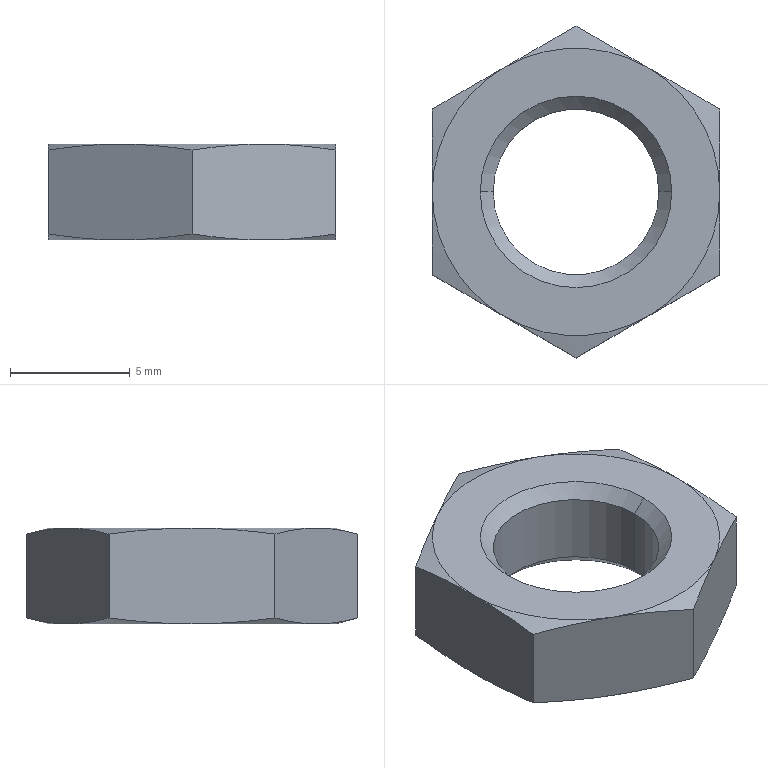Part | SolidWorks | features BaseBody 1 | 1 solid | 26 faces | box 12 x 13.856 x 4 mm | volume 340.073 mm3 | cone 16 | plane 8 | cylinder 2 | commonest cylinder face diameters 6.917 x2
STEP:
#1=CARTESIAN_POINT('',(3.459,0.,0.5415));
#2=VERTEX_POINT('',#1);
#3=CARTESIAN_POINT('',(-3.459,0.,0.5415));
#4=VERTEX_POINT('',#3);
#5=CARTESIAN_POINT('',(0.,0.,0.5415));
#6=DIRECTION('',(0.,0.,-1.));
#7=DIRECTION('',(-1.,0.,0.));
#8=AXIS2_PLACEMENT_3D('',#5,#6,#7);
#9=CIRCLE('',#8,3.459);
#10=EDGE_CURVE('',#2,#4,#9,.T.);
#11=ORIENTED_EDGE('',*,*,#10,.F.);
#12=CARTESIAN_POINT('',(4.,0.,0.));
#13=VERTEX_POINT('',#12);
#14=CARTESIAN_POINT('',(3.459,0.,0.5415));
#15=DIRECTION('',(0.7071,0.,-0.7071));
#16=VECTOR('',#15,1000.);
#17=LINE('',#14,#16);
#18=EDGE_CURVE('',#2,#13,#17,.T.);
#19=ORIENTED_EDGE('',*,*,#18,.T.);
#20=CARTESIAN_POINT('',(-4.,0.,0.));
#21=VERTEX_POINT('',#20);
#22=CARTESIAN_POINT('',(0.,0.,0.));
#23=DIRECTION('',(0.,0.,-1.));
#24=DIRECTION('',(-1.,0.,0.));
#25=AXIS2_PLACEMENT_3D('',#22,#23,#24);
#26=CIRCLE('',#25,4.);
#27=EDGE_CURVE('',#13,#21,#26,.T.);
#28=ORIENTED_EDGE('',*,*,#27,.T.);
#29=CARTESIAN_POINT('',(-3.459,0.,0.5415));
#30=DIRECTION('',(-0.7071,0.,-0.7071));
#31=VECTOR('',#30,1000.);
#32=LINE('',#29,#31);
#33=EDGE_CURVE('',#4,#21,#32,.T.);
#34=ORIENTED_EDGE('',*,*,#33,.F.);
#35=EDGE_LOOP('',(#11,#19,#28,#34));
#36=FACE_OUTER_BOUND('',#35,.T.);
#37=CARTESIAN_POINT('',(0.,0.,0.5415));
#38=DIRECTION('',(0.,0.,-1.));
#39=DIRECTION('',(-1.,0.,0.));
#40=AXIS2_PLACEMENT_3D('',#37,#38,#39);
#41=CONICAL_SURFACE('',#40,3.459,0.7854);
#42=ADVANCED_FACE('',(#36),#41,.F.);
#43=CARTESIAN_POINT('',(3.459,0.,3.459));
#44=VERTEX_POINT('',#43);
#45=CARTESIAN_POINT('',(-3.459,0.,3.459));
#46=VERTEX_POINT('',#45);
#47=CARTESIAN_POINT('',(0.,0.,3.459));
#48=DIRECTION('',(0.,0.,-1.));
#49=DIRECTION('',(-1.,0.,0.));
#50=AXIS2_PLACEMENT_3D('',#47,#48,#49);
#51=CIRCLE('',#50,3.459);
#52=EDGE_CURVE('',#44,#46,#51,.T.);
#53=ORIENTED_EDGE('',*,*,#52,.F.);
#54=CARTESIAN_POINT('',(3.459,0.,0.));
#55=DIRECTION('',(0.,0.,-1.));
#56=VECTOR('',#55,1000.);
#57=LINE('',#54,#56);
#58=EDGE_CURVE('',#44,#2,#57,.T.);
#59=ORIENTED_EDGE('',*,*,#58,.T.);
#60=ORIENTED_EDGE('',*,*,#10,.T.);
#61=CARTESIAN_POINT('',(-3.459,0.,0.));
#62=DIRECTION('',(0.,0.,-1.));
#63=VECTOR('',#62,1000.);
#64=LINE('',#61,#63);
#65=EDGE_CURVE('',#46,#4,#64,.T.);
#66=ORIENTED_EDGE('',*,*,#65,.F.);
#67=EDGE_LOOP('',(#53,#59,#60,#66));
#68=FACE_OUTER_BOUND('',#67,.T.);
#69=CARTESIAN_POINT('',(0.,0.,0.));
#70=DIRECTION('',(0.,0.,-1.));
#71=DIRECTION('',(-1.,0.,0.));
#72=AXIS2_PLACEMENT_3D('',#69,#70,#71);
#73=CYLINDRICAL_SURFACE('',#72,3.459);
#74=ADVANCED_FACE('',(#68),#73,.F.);
#75=ORIENTED_EDGE('',*,*,#52,.T.);
#76=CARTESIAN_POINT('',(-4.,0.,4.));
#77=VERTEX_POINT('',#76);
#78=CARTESIAN_POINT('',(-4.,0.,4.));
#79=DIRECTION('',(-0.7071,0.,0.7071));
#80=VECTOR('',#79,1000.);
#81=LINE('',#78,#80);
#82=EDGE_CURVE('',#46,#77,#81,.T.);
#83=ORIENTED_EDGE('',*,*,#82,.T.);
#84=CARTESIAN_POINT('',(4.,0.,4.));
#85=VERTEX_POINT('',#84);
#86=CARTESIAN_POINT('',(0.,0.,4.));
#87=DIRECTION('',(0.,0.,-1.));
#88=DIRECTION('',(-1.,0.,0.));
#89=AXIS2_PLACEMENT_3D('',#86,#87,#88);
#90=CIRCLE('',#89,4.);
#91=EDGE_CURVE('',#85,#77,#90,.T.);
#92=ORIENTED_EDGE('',*,*,#91,.F.);
#93=CARTESIAN_POINT('',(4.,0.,4.));
#94=DIRECTION('',(0.7071,0.,0.7071));
#95=VECTOR('',#94,1000.);
#96=LINE('',#93,#95);
#97=EDGE_CURVE('',#44,#85,#96,.T.);
#98=ORIENTED_EDGE('',*,*,#97,.F.);
#99=EDGE_LOOP('',(#75,#83,#92,#98));
#100=FACE_OUTER_BOUND('',#99,.T.);
#101=CARTESIAN_POINT('',(0.,0.,4.));
#102=DIRECTION('',(0.,0.,1.));
#103=DIRECTION('',(1.,0.,0.));
#104=AXIS2_PLACEMENT_3D('',#101,#102,#103);
#105=CONICAL_SURFACE('',#104,4.,0.7854);
#106=ADVANCED_FACE('',(#100),#105,.F.);
#107=CARTESIAN_POINT('',(-6.,-3.464,3.751));
#108=VERTEX_POINT('',#107);
#109=CARTESIAN_POINT('',(-6.,0.,4.));
#110=VERTEX_POINT('',#109);
#111=CARTESIAN_POINT('',(-6.,-3.464,3.751));
#112=CARTESIAN_POINT('',(-6.,-2.891,3.828));
#113=CARTESIAN_POINT('',(-6.,-2.318,3.891));
#114=CARTESIAN_POINT('',(-6.,-1.162,3.977));
#115=CARTESIAN_POINT('',(-6.,-0.5807,4.));
#116=CARTESIAN_POINT('',(-6.,0.,4.));
#117=B_SPLINE_CURVE_WITH_KNOTS('',3,(#111,#112,#113,#114,#115,#116),.UNSPECIFIED.,.F.,.F.,(4,2,4),(7.335,9.068,10.801),.UNSPECIFIED.);
#118=EDGE_CURVE('',#108,#110,#117,.T.);
#119=ORIENTED_EDGE('',*,*,#118,.F.);
#120=CARTESIAN_POINT('',(-3.,-5.196,4.));
#121=VERTEX_POINT('',#120);
#122=CARTESIAN_POINT('',(-3.,-5.196,4.));
#123=CARTESIAN_POINT('',(-3.501,-4.907,4.));
#124=CARTESIAN_POINT('',(-4.,-4.619,3.977));
#125=CARTESIAN_POINT('',(-5.001,-4.041,3.891));
#126=CARTESIAN_POINT('',(-5.502,-3.752,3.828));
#127=CARTESIAN_POINT('',(-6.,-3.464,3.751));
#128=B_SPLINE_CURVE_WITH_KNOTS('',3,(#122,#123,#124,#125,#126,#127),.UNSPECIFIED.,.F.,.F.,(4,2,4),(3.464,5.196,6.928),.UNSPECIFIED.);
#129=EDGE_CURVE('',#121,#108,#128,.T.);
#130=ORIENTED_EDGE('',*,*,#129,.F.);
#131=CARTESIAN_POINT('',(0.,0.,4.));
#132=DIRECTION('',(0.,0.,-1.));
#133=DIRECTION('',(-0.5,-0.866,0.));
#134=AXIS2_PLACEMENT_3D('',#131,#132,#133);
#135=CIRCLE('',#134,6.);
#136=EDGE_CURVE('',#121,#110,#135,.T.);
#137=ORIENTED_EDGE('',*,*,#136,.T.);
#138=EDGE_LOOP('',(#119,#130,#137));
#139=FACE_OUTER_BOUND('',#138,.T.);
#140=CARTESIAN_POINT('',(0.,0.,2.));
#141=DIRECTION('',(0.,0.,-1.));
#142=DIRECTION('',(-1.,0.,0.));
#143=AXIS2_PLACEMENT_3D('',#140,#141,#142);
#144=CONICAL_SURFACE('',#143,13.464,1.309);
#145=ADVANCED_FACE('',(#139),#144,.T.);
#146=ORIENTED_EDGE('',*,*,#118,.T.);
#147=CARTESIAN_POINT('',(-6.,3.464,3.751));
#148=VERTEX_POINT('',#147);
#149=CARTESIAN_POINT('',(-6.,0.,4.));
#150=CARTESIAN_POINT('',(-6.,0.5782,4.));
#151=CARTESIAN_POINT('',(-6.,1.154,3.977));
#152=CARTESIAN_POINT('',(-6.,2.31,3.891));
#153=CARTESIAN_POINT('',(-6.,2.889,3.828));
#154=CARTESIAN_POINT('',(-6.,3.464,3.751));
#155=B_SPLINE_CURVE_WITH_KNOTS('',3,(#149,#150,#151,#152,#153,#154),.UNSPECIFIED.,.F.,.F.,(4,2,4),(10.801,12.511,14.221),.UNSPECIFIED.);
#156=EDGE_CURVE('',#110,#148,#155,.T.);
#157=ORIENTED_EDGE('',*,*,#156,.T.);
#158=CARTESIAN_POINT('',(-6.,3.464,0.2487));
#159=VERTEX_POINT('',#158);
#160=CARTESIAN_POINT('',(-6.,3.464,3.751));
#161=DIRECTION('',(0.,0.,-1.));
#162=VECTOR('',#161,1000.);
#163=LINE('',#160,#162);
#164=EDGE_CURVE('',#148,#159,#163,.T.);
#165=ORIENTED_EDGE('',*,*,#164,.T.);
#166=CARTESIAN_POINT('',(-6.,0.,0.));
#167=VERTEX_POINT('',#166);
#168=CARTESIAN_POINT('',(-6.,3.464,0.2487));
#169=CARTESIAN_POINT('',(-6.,2.891,0.1719));
#170=CARTESIAN_POINT('',(-6.,2.318,0.1093));
#171=CARTESIAN_POINT('',(-6.,1.162,0.0231));
#172=CARTESIAN_POINT('',(-6.,0.5807,0.00000014));
#173=CARTESIAN_POINT('',(-6.,0.,0.));
#174=B_SPLINE_CURVE_WITH_KNOTS('',3,(#168,#169,#170,#171,#172,#173),.UNSPECIFIED.,.F.,.F.,(4,2,4),(7.335,9.068,10.801),.UNSPECIFIED.);
#175=EDGE_CURVE('',#159,#167,#174,.T.);
#176=ORIENTED_EDGE('',*,*,#175,.T.);
#177=CARTESIAN_POINT('',(-6.,-3.464,0.2487));
#178=VERTEX_POINT('',#177);
#179=CARTESIAN_POINT('',(-6.,0.,0.));
#180=CARTESIAN_POINT('',(-6.,-0.5782,-0.00000014));
#181=CARTESIAN_POINT('',(-6.,-1.154,0.02271));
#182=CARTESIAN_POINT('',(-6.,-2.31,0.1086));
#183=CARTESIAN_POINT('',(-6.,-2.889,0.1716));
#184=CARTESIAN_POINT('',(-6.,-3.464,0.2487));
#185=B_SPLINE_CURVE_WITH_KNOTS('',3,(#179,#180,#181,#182,#183,#184),.UNSPECIFIED.,.F.,.F.,(4,2,4),(10.801,12.511,14.221),.UNSPECIFIED.);
#186=EDGE_CURVE('',#167,#178,#185,.T.);
#187=ORIENTED_EDGE('',*,*,#186,.T.);
#188=CARTESIAN_POINT('',(-6.,-3.464,3.751));
#189=DIRECTION('',(0.,0.,-1.));
#190=VECTOR('',#189,1000.);
#191=LINE('',#188,#190);
#192=EDGE_CURVE('',#108,#178,#191,.T.);
#193=ORIENTED_EDGE('',*,*,#192,.F.);
#194=EDGE_LOOP('',(#146,#157,#165,#176,#187,#193));
#195=FACE_OUTER_BOUND('',#194,.T.);
#196=CARTESIAN_POINT('',(-6.,3.464,4.));
#197=DIRECTION('',(1.,0.,0.));
#198=DIRECTION('',(0.,0.,-1.));
#199=AXIS2_PLACEMENT_3D('',#196,#197,#198);
#200=PLANE('',#199);
#201=ADVANCED_FACE('',(#195),#200,.F.);
#202=CARTESIAN_POINT('',(0.,-6.928,3.751));
#203=VERTEX_POINT('',#202);
#204=CARTESIAN_POINT('',(0.,-6.928,3.751));
#205=CARTESIAN_POINT('',(-0.4983,-6.64,3.828));
#206=CARTESIAN_POINT('',(-0.9989,-6.351,3.891));
#207=CARTESIAN_POINT('',(-2.,-5.774,3.977));
#208=CARTESIAN_POINT('',(-2.499,-5.485,4.));
#209=CARTESIAN_POINT('',(-3.,-5.196,4.));
#210=B_SPLINE_CURVE_WITH_KNOTS('',3,(#204,#205,#206,#207,#208,#209),.UNSPECIFIED.,.F.,.F.,(4,2,4),(0.0002309,1.732,3.464),.UNSPECIFIED.);
#211=EDGE_CURVE('',#203,#121,#210,.T.);
#212=ORIENTED_EDGE('',*,*,#211,.T.);
#213=ORIENTED_EDGE('',*,*,#129,.T.);
#214=ORIENTED_EDGE('',*,*,#192,.T.);
#215=CARTESIAN_POINT('',(-3.,-5.196,0.));
#216=VERTEX_POINT('',#215);
#217=CARTESIAN_POINT('',(-6.,-3.464,0.2487));
#218=CARTESIAN_POINT('',(-5.502,-3.752,0.1716));
#219=CARTESIAN_POINT('',(-5.001,-4.041,0.1087));
#220=CARTESIAN_POINT('',(-4.,-4.619,0.02273));
#221=CARTESIAN_POINT('',(-3.501,-4.907,0.));
#222=CARTESIAN_POINT('',(-3.,-5.196,0.));
#223=B_SPLINE_CURVE_WITH_KNOTS('',3,(#217,#218,#219,#220,#221,#222),.UNSPECIFIED.,.F.,.F.,(4,2,4),(0.0002309,1.732,3.464),.UNSPECIFIED.);
#224=EDGE_CURVE('',#178,#216,#223,.T.);
#225=ORIENTED_EDGE('',*,*,#224,.T.);
#226=CARTESIAN_POINT('',(0.,-6.928,0.2487));
#227=VERTEX_POINT('',#226);
#228=CARTESIAN_POINT('',(-3.,-5.196,0.));
#229=CARTESIAN_POINT('',(-2.499,-5.485,0.));
#230=CARTESIAN_POINT('',(-2.,-5.774,0.02273));
#231=CARTESIAN_POINT('',(-0.9989,-6.351,0.1087));
#232=CARTESIAN_POINT('',(-0.4983,-6.64,0.1716));
#233=CARTESIAN_POINT('',(0.,-6.928,0.2487));
#234=B_SPLINE_CURVE_WITH_KNOTS('',3,(#228,#229,#230,#231,#232,#233),.UNSPECIFIED.,.F.,.F.,(4,2,4),(3.464,5.196,6.928),.UNSPECIFIED.);
#235=EDGE_CURVE('',#216,#227,#234,.T.);
#236=ORIENTED_EDGE('',*,*,#235,.T.);
#237=CARTESIAN_POINT('',(0.,-6.928,3.751));
#238=DIRECTION('',(0.,0.,-1.));
#239=VECTOR('',#238,1000.);
#240=LINE('',#237,#239);
#241=EDGE_CURVE('',#203,#227,#240,.T.);
#242=ORIENTED_EDGE('',*,*,#241,.F.);
#243=EDGE_LOOP('',(#212,#213,#214,#225,#236,#242));
#244=FACE_OUTER_BOUND('',#243,.T.);
#245=CARTESIAN_POINT('',(-6.,-3.464,4.));
#246=DIRECTION('',(0.5,0.866,0.));
#247=DIRECTION('',(-0.866,0.5,0.));
#248=AXIS2_PLACEMENT_3D('',#245,#246,#247);
#249=PLANE('',#248);
#250=ADVANCED_FACE('',(#244),#249,.F.);
#251=ORIENTED_EDGE('',*,*,#91,.T.);
#252=CARTESIAN_POINT('',(0.,0.,4.));
#253=DIRECTION('',(0.,0.,-1.));
#254=DIRECTION('',(-1.,0.,0.));
#255=AXIS2_PLACEMENT_3D('',#252,#253,#254);
#256=CIRCLE('',#255,4.);
#257=EDGE_CURVE('',#77,#85,#256,.T.);
#258=ORIENTED_EDGE('',*,*,#257,.T.);
#259=EDGE_LOOP('',(#251,#258));
#260=FACE_BOUND('',#259,.T.);
#261=CARTESIAN_POINT('',(-3.,5.196,4.));
#262=VERTEX_POINT('',#261);
#263=CARTESIAN_POINT('',(3.,5.196,4.));
#264=VERTEX_POINT('',#263);
#265=CARTESIAN_POINT('',(0.,0.,4.));
#266=DIRECTION('',(0.,0.,-1.));
#267=DIRECTION('',(-0.5,0.866,0.));
#268=AXIS2_PLACEMENT_3D('',#265,#266,#267);
#269=CIRCLE('',#268,6.);
#270=EDGE_CURVE('',#262,#264,#269,.T.);
#271=ORIENTED_EDGE('',*,*,#270,.F.);
#272=CARTESIAN_POINT('',(0.,0.,4.));
#273=DIRECTION('',(0.,0.,-1.));
#274=DIRECTION('',(-1.,0.,0.));
#275=AXIS2_PLACEMENT_3D('',#272,#273,#274);
#276=CIRCLE('',#275,6.);
#277=EDGE_CURVE('',#110,#262,#276,.T.);
#278=ORIENTED_EDGE('',*,*,#277,.F.);
#279=ORIENTED_EDGE('',*,*,#136,.F.);
#280=CARTESIAN_POINT('',(3.,-5.196,4.));
#281=VERTEX_POINT('',#280);
#282=CARTESIAN_POINT('',(0.,0.,4.));
#283=DIRECTION('',(0.,0.,-1.));
#284=DIRECTION('',(0.5,-0.866,0.));
#285=AXIS2_PLACEMENT_3D('',#282,#283,#284);
#286=CIRCLE('',#285,6.);
#287=EDGE_CURVE('',#281,#121,#286,.T.);
#288=ORIENTED_EDGE('',*,*,#287,.F.);
#289=CARTESIAN_POINT('',(6.,0.,4.));
#290=VERTEX_POINT('',#289);
#291=CARTESIAN_POINT('',(0.,0.,4.));
#292=DIRECTION('',(0.,0.,-1.));
#293=DIRECTION('',(1.,0.,0.));
#294=AXIS2_PLACEMENT_3D('',#291,#292,#293);
#295=CIRCLE('',#294,6.);
#296=EDGE_CURVE('',#290,#281,#295,.T.);
#297=ORIENTED_EDGE('',*,*,#296,.F.);
#298=CARTESIAN_POINT('',(0.,0.,4.));
#299=DIRECTION('',(0.,0.,-1.));
#300=DIRECTION('',(0.5,0.866,0.));
#301=AXIS2_PLACEMENT_3D('',#298,#299,#300);
#302=CIRCLE('',#301,6.);
#303=EDGE_CURVE('',#264,#290,#302,.T.);
#304=ORIENTED_EDGE('',*,*,#303,.F.);
#305=EDGE_LOOP('',(#271,#278,#279,#288,#297,#304));
#306=FACE_OUTER_BOUND('',#305,.T.);
#307=CARTESIAN_POINT('',(0.,6.,4.));
#308=DIRECTION('',(0.,0.,1.));
#309=DIRECTION('',(1.,0.,0.));
#310=AXIS2_PLACEMENT_3D('',#307,#308,#309);
#311=PLANE('',#310);
#312=ADVANCED_FACE('',(#260,#306),#311,.T.);
#313=ORIENTED_EDGE('',*,*,#156,.F.);
#314=ORIENTED_EDGE('',*,*,#277,.T.);
#315=CARTESIAN_POINT('',(-6.,3.464,3.751));
#316=CARTESIAN_POINT('',(-5.502,3.752,3.828));
#317=CARTESIAN_POINT('',(-5.001,4.041,3.891));
#318=CARTESIAN_POINT('',(-4.,4.619,3.977));
#319=CARTESIAN_POINT('',(-3.501,4.907,4.));
#320=CARTESIAN_POINT('',(-3.,5.196,4.));
#321=B_SPLINE_CURVE_WITH_KNOTS('',3,(#315,#316,#317,#318,#319,#320),.UNSPECIFIED.,.F.,.F.,(4,2,4),(0.0002309,1.732,3.464),.UNSPECIFIED.);
#322=EDGE_CURVE('',#148,#262,#321,.T.);
#323=ORIENTED_EDGE('',*,*,#322,.F.);
#324=EDGE_LOOP('',(#313,#314,#323));
#325=FACE_OUTER_BOUND('',#324,.T.);
#326=CARTESIAN_POINT('',(0.,0.,2.));
#327=DIRECTION('',(0.,0.,-1.));
#328=DIRECTION('',(-1.,0.,0.));
#329=AXIS2_PLACEMENT_3D('',#326,#327,#328);
#330=CONICAL_SURFACE('',#329,13.464,1.309);
#331=ADVANCED_FACE('',(#325),#330,.T.);
#332=ORIENTED_EDGE('',*,*,#322,.T.);
#333=CARTESIAN_POINT('',(0.,6.928,3.751));
#334=VERTEX_POINT('',#333);
#335=CARTESIAN_POINT('',(-3.,5.196,4.));
#336=CARTESIAN_POINT('',(-2.499,5.485,4.));
#337=CARTESIAN_POINT('',(-2.,5.774,3.977));
#338=CARTESIAN_POINT('',(-0.9989,6.351,3.891));
#339=CARTESIAN_POINT('',(-0.4983,6.64,3.828));
#340=CARTESIAN_POINT('',(0.,6.928,3.751));
#341=B_SPLINE_CURVE_WITH_KNOTS('',3,(#335,#336,#337,#338,#339,#340),.UNSPECIFIED.,.F.,.F.,(4,2,4),(3.464,5.196,6.928),.UNSPECIFIED.);
#342=EDGE_CURVE('',#262,#334,#341,.T.);
#343=ORIENTED_EDGE('',*,*,#342,.T.);
#344=CARTESIAN_POINT('',(0.,6.928,0.2487));
#345=VERTEX_POINT('',#344);
#346=CARTESIAN_POINT('',(0.,6.928,3.751));
#347=DIRECTION('',(0.,0.,-1.));
#348=VECTOR('',#347,1000.);
#349=LINE('',#346,#348);
#350=EDGE_CURVE('',#334,#345,#349,.T.);
#351=ORIENTED_EDGE('',*,*,#350,.T.);
#352=CARTESIAN_POINT('',(-3.,5.196,0.));
#353=VERTEX_POINT('',#352);
#354=CARTESIAN_POINT('',(0.,6.928,0.2487));
#355=CARTESIAN_POINT('',(-0.4983,6.64,0.1716));
#356=CARTESIAN_POINT('',(-0.9989,6.351,0.1087));
#357=CARTESIAN_POINT('',(-2.,5.774,0.02273));
#358=CARTESIAN_POINT('',(-2.499,5.485,0.));
#359=CARTESIAN_POINT('',(-3.,5.196,0.));
#360=B_SPLINE_CURVE_WITH_KNOTS('',3,(#354,#355,#356,#357,#358,#359),.UNSPECIFIED.,.F.,.F.,(4,2,4),(0.0002309,1.732,3.464),.UNSPECIFIED.);
#361=EDGE_CURVE('',#345,#353,#360,.T.);
#362=ORIENTED_EDGE('',*,*,#361,.T.);
#363=CARTESIAN_POINT('',(-3.,5.196,0.));
#364=CARTESIAN_POINT('',(-3.501,4.907,0.));
#365=CARTESIAN_POINT('',(-4.,4.619,0.02273));
#366=CARTESIAN_POINT('',(-5.001,4.041,0.1087));
#367=CARTESIAN_POINT('',(-5.502,3.752,0.1716));
#368=CARTESIAN_POINT('',(-6.,3.464,0.2487));
#369=B_SPLINE_CURVE_WITH_KNOTS('',3,(#363,#364,#365,#366,#367,#368),.UNSPECIFIED.,.F.,.F.,(4,2,4),(3.464,5.196,6.928),.UNSPECIFIED.);
#370=EDGE_CURVE('',#353,#159,#369,.T.);
#371=ORIENTED_EDGE('',*,*,#370,.T.);
#372=ORIENTED_EDGE('',*,*,#164,.F.);
#373=EDGE_LOOP('',(#332,#343,#351,#362,#371,#372));
#374=FACE_OUTER_BOUND('',#373,.T.);
#375=CARTESIAN_POINT('',(0.,6.928,4.));
#376=DIRECTION('',(0.5,-0.866,0.));
#377=DIRECTION('',(0.866,0.5,0.));
#378=AXIS2_PLACEMENT_3D('',#375,#376,#377);
#379=PLANE('',#378);
#380=ADVANCED_FACE('',(#374),#379,.F.);
#381=ORIENTED_EDGE('',*,*,#370,.F.);
#382=CARTESIAN_POINT('',(0.,0.,0.));
#383=DIRECTION('',(0.,0.,-1.));
#384=DIRECTION('',(-1.,0.,0.));
#385=AXIS2_PLACEMENT_3D('',#382,#383,#384);
#386=CIRCLE('',#385,6.);
#387=EDGE_CURVE('',#167,#353,#386,.T.);
#388=ORIENTED_EDGE('',*,*,#387,.F.);
#389=ORIENTED_EDGE('',*,*,#175,.F.);
#390=EDGE_LOOP('',(#381,#388,#389));
#391=FACE_OUTER_BOUND('',#390,.T.);
#392=CARTESIAN_POINT('',(0.,0.,0.));
#393=DIRECTION('',(0.,0.,1.));
#394=DIRECTION('',(1.,0.,0.));
#395=AXIS2_PLACEMENT_3D('',#392,#393,#394);
#396=CONICAL_SURFACE('',#395,6.,1.309);
#397=ADVANCED_FACE('',(#391),#396,.T.);
#398=ORIENTED_EDGE('',*,*,#186,.F.);
#399=CARTESIAN_POINT('',(0.,0.,0.));
#400=DIRECTION('',(0.,0.,-1.));
#401=DIRECTION('',(-0.5,-0.866,0.));
#402=AXIS2_PLACEMENT_3D('',#399,#400,#401);
#403=CIRCLE('',#402,6.);
#404=EDGE_CURVE('',#216,#167,#403,.T.);
#405=ORIENTED_EDGE('',*,*,#404,.F.);
#406=ORIENTED_EDGE('',*,*,#224,.F.);
#407=EDGE_LOOP('',(#398,#405,#406));
#408=FACE_OUTER_BOUND('',#407,.T.);
#409=CARTESIAN_POINT('',(0.,0.,0.));
#410=DIRECTION('',(0.,0.,1.));
#411=DIRECTION('',(1.,0.,0.));
#412=AXIS2_PLACEMENT_3D('',#409,#410,#411);
#413=CONICAL_SURFACE('',#412,6.,1.309);
#414=ADVANCED_FACE('',(#408),#413,.T.);
#415=CARTESIAN_POINT('',(3.,-5.196,4.));
#416=CARTESIAN_POINT('',(2.499,-5.485,4.));
#417=CARTESIAN_POINT('',(2.,-5.774,3.977));
#418=CARTESIAN_POINT('',(0.9989,-6.351,3.891));
#419=CARTESIAN_POINT('',(0.4983,-6.64,3.828));
#420=CARTESIAN_POINT('',(0.,-6.928,3.751));
#421=B_SPLINE_CURVE_WITH_KNOTS('',3,(#415,#416,#417,#418,#419,#420),.UNSPECIFIED.,.F.,.F.,(4,2,4),(3.464,5.196,6.928),.UNSPECIFIED.);
#422=EDGE_CURVE('',#281,#203,#421,.T.);
#423=ORIENTED_EDGE('',*,*,#422,.F.);
#424=ORIENTED_EDGE('',*,*,#287,.T.);
#425=ORIENTED_EDGE('',*,*,#211,.F.);
#426=EDGE_LOOP('',(#423,#424,#425));
#427=FACE_OUTER_BOUND('',#426,.T.);
#428=CARTESIAN_POINT('',(0.,0.,2.));
#429=DIRECTION('',(0.,0.,-1.));
#430=DIRECTION('',(-1.,0.,0.));
#431=AXIS2_PLACEMENT_3D('',#428,#429,#430);
#432=CONICAL_SURFACE('',#431,13.464,1.309);
#433=ADVANCED_FACE('',(#427),#432,.T.);
#434=CARTESIAN_POINT('',(3.,-5.196,0.));
#435=VERTEX_POINT('',#434);
#436=CARTESIAN_POINT('',(0.,-6.928,0.2487));
#437=CARTESIAN_POINT('',(0.4983,-6.64,0.1716));
#438=CARTESIAN_POINT('',(0.9989,-6.351,0.1087));
#439=CARTESIAN_POINT('',(2.,-5.774,0.02273));
#440=CARTESIAN_POINT('',(2.499,-5.485,0.));
#441=CARTESIAN_POINT('',(3.,-5.196,0.));
#442=B_SPLINE_CURVE_WITH_KNOTS('',3,(#436,#437,#438,#439,#440,#441),.UNSPECIFIED.,.F.,.F.,(4,2,4),(0.0002309,1.732,3.464),.UNSPECIFIED.);
#443=EDGE_CURVE('',#227,#435,#442,.T.);
#444=ORIENTED_EDGE('',*,*,#443,.F.);
#445=ORIENTED_EDGE('',*,*,#235,.F.);
#446=CARTESIAN_POINT('',(0.,0.,0.));
#447=DIRECTION('',(0.,0.,-1.));
#448=DIRECTION('',(0.5,-0.866,0.));
#449=AXIS2_PLACEMENT_3D('',#446,#447,#448);
#450=CIRCLE('',#449,6.);
#451=EDGE_CURVE('',#435,#216,#450,.T.);
#452=ORIENTED_EDGE('',*,*,#451,.F.);
#453=EDGE_LOOP('',(#444,#445,#452));
#454=FACE_OUTER_BOUND('',#453,.T.);
#455=CARTESIAN_POINT('',(0.,0.,0.));
#456=DIRECTION('',(0.,0.,1.));
#457=DIRECTION('',(1.,0.,0.));
#458=AXIS2_PLACEMENT_3D('',#455,#456,#457);
#459=CONICAL_SURFACE('',#458,6.,1.309);
#460=ADVANCED_FACE('',(#454),#459,.T.);
#461=CARTESIAN_POINT('',(6.,-3.464,3.751));
#462=VERTEX_POINT('',#461);
#463=CARTESIAN_POINT('',(6.,-3.464,3.751));
#464=CARTESIAN_POINT('',(5.502,-3.752,3.828));
#465=CARTESIAN_POINT('',(5.001,-4.041,3.891));
#466=CARTESIAN_POINT('',(4.,-4.619,3.977));
#467=CARTESIAN_POINT('',(3.501,-4.907,4.));
#468=CARTESIAN_POINT('',(3.,-5.196,4.));
#469=B_SPLINE_CURVE_WITH_KNOTS('',3,(#463,#464,#465,#466,#467,#468),.UNSPECIFIED.,.F.,.F.,(4,2,4),(0.0002309,1.732,3.464),.UNSPECIFIED.);
#470=EDGE_CURVE('',#462,#281,#469,.T.);
#471=ORIENTED_EDGE('',*,*,#470,.T.);
#472=ORIENTED_EDGE('',*,*,#422,.T.);
#473=ORIENTED_EDGE('',*,*,#241,.T.);
#474=ORIENTED_EDGE('',*,*,#443,.T.);
#475=CARTESIAN_POINT('',(6.,-3.464,0.2487));
#476=VERTEX_POINT('',#475);
#477=CARTESIAN_POINT('',(3.,-5.196,0.));
#478=CARTESIAN_POINT('',(3.501,-4.907,0.));
#479=CARTESIAN_POINT('',(4.,-4.619,0.02273));
#480=CARTESIAN_POINT('',(5.001,-4.041,0.1087));
#481=CARTESIAN_POINT('',(5.502,-3.752,0.1716));
#482=CARTESIAN_POINT('',(6.,-3.464,0.2487));
#483=B_SPLINE_CURVE_WITH_KNOTS('',3,(#477,#478,#479,#480,#481,#482),.UNSPECIFIED.,.F.,.F.,(4,2,4),(3.464,5.196,6.928),.UNSPECIFIED.);
#484=EDGE_CURVE('',#435,#476,#483,.T.);
#485=ORIENTED_EDGE('',*,*,#484,.T.);
#486=CARTESIAN_POINT('',(6.,-3.464,3.751));
#487=DIRECTION('',(0.,0.,-1.));
#488=VECTOR('',#487,1000.);
#489=LINE('',#486,#488);
#490=EDGE_CURVE('',#462,#476,#489,.T.);
#491=ORIENTED_EDGE('',*,*,#490,.F.);
#492=EDGE_LOOP('',(#471,#472,#473,#474,#485,#491));
#493=FACE_OUTER_BOUND('',#492,.T.);
#494=CARTESIAN_POINT('',(0.,-6.928,4.));
#495=DIRECTION('',(-0.5,0.866,0.));
#496=DIRECTION('',(-0.866,-0.5,0.));
#497=AXIS2_PLACEMENT_3D('',#494,#495,#496);
#498=PLANE('',#497);
#499=ADVANCED_FACE('',(#493),#498,.F.);
#500=ORIENTED_EDGE('',*,*,#82,.F.);
#501=CARTESIAN_POINT('',(0.,0.,3.459));
#502=DIRECTION('',(0.,0.,-1.));
#503=DIRECTION('',(-1.,0.,0.));
#504=AXIS2_PLACEMENT_3D('',#501,#502,#503);
#505=CIRCLE('',#504,3.459);
#506=EDGE_CURVE('',#46,#44,#505,.T.);
#507=ORIENTED_EDGE('',*,*,#506,.T.);
#508=ORIENTED_EDGE('',*,*,#97,.T.);
#509=ORIENTED_EDGE('',*,*,#257,.F.);
#510=EDGE_LOOP('',(#500,#507,#508,#509));
#511=FACE_OUTER_BOUND('',#510,.T.);
#512=CARTESIAN_POINT('',(0.,0.,4.));
#513=DIRECTION('',(0.,0.,1.));
#514=DIRECTION('',(1.,0.,0.));
#515=AXIS2_PLACEMENT_3D('',#512,#513,#514);
#516=CONICAL_SURFACE('',#515,4.,0.7854);
#517=ADVANCED_FACE('',(#511),#516,.F.);
#518=CARTESIAN_POINT('',(0.,6.928,3.751));
#519=CARTESIAN_POINT('',(0.4983,6.64,3.828));
#520=CARTESIAN_POINT('',(0.9989,6.351,3.891));
#521=CARTESIAN_POINT('',(2.,5.774,3.977));
#522=CARTESIAN_POINT('',(2.499,5.485,4.));
#523=CARTESIAN_POINT('',(3.,5.196,4.));
#524=B_SPLINE_CURVE_WITH_KNOTS('',3,(#518,#519,#520,#521,#522,#523),.UNSPECIFIED.,.F.,.F.,(4,2,4),(0.0002309,1.732,3.464),.UNSPECIFIED.);
#525=EDGE_CURVE('',#334,#264,#524,.T.);
#526=ORIENTED_EDGE('',*,*,#525,.F.);
#527=ORIENTED_EDGE('',*,*,#342,.F.);
#528=ORIENTED_EDGE('',*,*,#270,.T.);
#529=EDGE_LOOP('',(#526,#527,#528));
#530=FACE_OUTER_BOUND('',#529,.T.);
#531=CARTESIAN_POINT('',(0.,0.,2.));
#532=DIRECTION('',(0.,0.,-1.));
#533=DIRECTION('',(-1.,0.,0.));
#534=AXIS2_PLACEMENT_3D('',#531,#532,#533);
#535=CONICAL_SURFACE('',#534,13.464,1.309);
#536=ADVANCED_FACE('',(#530),#535,.T.);
#537=CARTESIAN_POINT('',(6.,0.,4.));
#538=CARTESIAN_POINT('',(6.,-0.5782,4.));
#539=CARTESIAN_POINT('',(6.,-1.154,3.977));
#540=CARTESIAN_POINT('',(6.,-2.31,3.891));
#541=CARTESIAN_POINT('',(6.,-2.889,3.828));
#542=CARTESIAN_POINT('',(6.,-3.464,3.751));
#543=B_SPLINE_CURVE_WITH_KNOTS('',3,(#537,#538,#539,#540,#541,#542),.UNSPECIFIED.,.F.,.F.,(4,2,4),(10.801,12.511,14.221),.UNSPECIFIED.);
#544=EDGE_CURVE('',#290,#462,#543,.T.);
#545=ORIENTED_EDGE('',*,*,#544,.F.);
#546=ORIENTED_EDGE('',*,*,#296,.T.);
#547=ORIENTED_EDGE('',*,*,#470,.F.);
#548=EDGE_LOOP('',(#545,#546,#547));
#549=FACE_OUTER_BOUND('',#548,.T.);
#550=CARTESIAN_POINT('',(0.,0.,2.));
#551=DIRECTION('',(0.,0.,-1.));
#552=DIRECTION('',(-1.,0.,0.));
#553=AXIS2_PLACEMENT_3D('',#550,#551,#552);
#554=CONICAL_SURFACE('',#553,13.464,1.309);
#555=ADVANCED_FACE('',(#549),#554,.T.);
#556=CARTESIAN_POINT('',(6.,3.464,3.751));
#557=VERTEX_POINT('',#556);
#558=CARTESIAN_POINT('',(3.,5.196,4.));
#559=CARTESIAN_POINT('',(3.501,4.907,4.));
#560=CARTESIAN_POINT('',(4.,4.619,3.977));
#561=CARTESIAN_POINT('',(5.001,4.041,3.891));
#562=CARTESIAN_POINT('',(5.502,3.752,3.828));
#563=CARTESIAN_POINT('',(6.,3.464,3.751));
#564=B_SPLINE_CURVE_WITH_KNOTS('',3,(#558,#559,#560,#561,#562,#563),.UNSPECIFIED.,.F.,.F.,(4,2,4),(3.464,5.196,6.928),.UNSPECIFIED.);
#565=EDGE_CURVE('',#264,#557,#564,.T.);
#566=ORIENTED_EDGE('',*,*,#565,.F.);
#567=ORIENTED_EDGE('',*,*,#303,.T.);
#568=CARTESIAN_POINT('',(6.,3.464,3.751));
#569=CARTESIAN_POINT('',(6.,2.891,3.828));
#570=CARTESIAN_POINT('',(6.,2.318,3.891));
#571=CARTESIAN_POINT('',(6.,1.162,3.977));
#572=CARTESIAN_POINT('',(6.,0.5807,4.));
#573=CARTESIAN_POINT('',(6.,0.,4.));
#574=B_SPLINE_CURVE_WITH_KNOTS('',3,(#568,#569,#570,#571,#572,#573),.UNSPECIFIED.,.F.,.F.,(4,2,4),(7.335,9.068,10.801),.UNSPECIFIED.);
#575=EDGE_CURVE('',#557,#290,#574,.T.);
#576=ORIENTED_EDGE('',*,*,#575,.F.);
#577=EDGE_LOOP('',(#566,#567,#576));
#578=FACE_OUTER_BOUND('',#577,.T.);
#579=CARTESIAN_POINT('',(0.,0.,2.));
#580=DIRECTION('',(0.,0.,-1.));
#581=DIRECTION('',(-1.,0.,0.));
#582=AXIS2_PLACEMENT_3D('',#579,#580,#581);
#583=CONICAL_SURFACE('',#582,13.464,1.309);
#584=ADVANCED_FACE('',(#578),#583,.T.);
#585=ORIENTED_EDGE('',*,*,#525,.T.);
#586=ORIENTED_EDGE('',*,*,#565,.T.);
#587=CARTESIAN_POINT('',(6.,3.464,0.2487));
#588=VERTEX_POINT('',#587);
#589=CARTESIAN_POINT('',(6.,3.464,3.751));
#590=DIRECTION('',(0.,0.,-1.));
#591=VECTOR('',#590,1000.);
#592=LINE('',#589,#591);
#593=EDGE_CURVE('',#557,#588,#592,.T.);
#594=ORIENTED_EDGE('',*,*,#593,.T.);
#595=CARTESIAN_POINT('',(3.,5.196,0.));
#596=VERTEX_POINT('',#595);
#597=CARTESIAN_POINT('',(6.,3.464,0.2487));
#598=CARTESIAN_POINT('',(5.502,3.752,0.1716));
#599=CARTESIAN_POINT('',(5.001,4.041,0.1087));
#600=CARTESIAN_POINT('',(4.,4.619,0.02273));
#601=CARTESIAN_POINT('',(3.501,4.907,0.));
#602=CARTESIAN_POINT('',(3.,5.196,0.));
#603=B_SPLINE_CURVE_WITH_KNOTS('',3,(#597,#598,#599,#600,#601,#602),.UNSPECIFIED.,.F.,.F.,(4,2,4),(0.0002309,1.732,3.464),.UNSPECIFIED.);
#604=EDGE_CURVE('',#588,#596,#603,.T.);
#605=ORIENTED_EDGE('',*,*,#604,.T.);
#606=CARTESIAN_POINT('',(3.,5.196,0.));
#607=CARTESIAN_POINT('',(2.499,5.485,0.));
#608=CARTESIAN_POINT('',(2.,5.774,0.02273));
#609=CARTESIAN_POINT('',(0.9989,6.351,0.1087));
#610=CARTESIAN_POINT('',(0.4983,6.64,0.1716));
#611=CARTESIAN_POINT('',(0.,6.928,0.2487));
#612=B_SPLINE_CURVE_WITH_KNOTS('',3,(#606,#607,#608,#609,#610,#611),.UNSPECIFIED.,.F.,.F.,(4,2,4),(3.464,5.196,6.928),.UNSPECIFIED.);
#613=EDGE_CURVE('',#596,#345,#612,.T.);
#614=ORIENTED_EDGE('',*,*,#613,.T.);
#615=ORIENTED_EDGE('',*,*,#350,.F.);
#616=EDGE_LOOP('',(#585,#586,#594,#605,#614,#615));
#617=FACE_OUTER_BOUND('',#616,.T.);
#618=CARTESIAN_POINT('',(6.,3.464,4.));
#619=DIRECTION('',(-0.5,-0.866,0.));
#620=DIRECTION('',(0.866,-0.5,0.));
#621=AXIS2_PLACEMENT_3D('',#618,#619,#620);
#622=PLANE('',#621);
#623=ADVANCED_FACE('',(#617),#622,.F.);
#624=ORIENTED_EDGE('',*,*,#361,.F.);
#625=ORIENTED_EDGE('',*,*,#613,.F.);
#626=CARTESIAN_POINT('',(0.,0.,0.));
#627=DIRECTION('',(0.,0.,-1.));
#628=DIRECTION('',(-0.5,0.866,0.));
#629=AXIS2_PLACEMENT_3D('',#626,#627,#628);
#630=CIRCLE('',#629,6.);
#631=EDGE_CURVE('',#353,#596,#630,.T.);
#632=ORIENTED_EDGE('',*,*,#631,.F.);
#633=EDGE_LOOP('',(#624,#625,#632));
#634=FACE_OUTER_BOUND('',#633,.T.);
#635=CARTESIAN_POINT('',(0.,0.,0.));
#636=DIRECTION('',(0.,0.,1.));
#637=DIRECTION('',(1.,0.,0.));
#638=AXIS2_PLACEMENT_3D('',#635,#636,#637);
#639=CONICAL_SURFACE('',#638,6.,1.309);
#640=ADVANCED_FACE('',(#634),#639,.T.);
#641=ORIENTED_EDGE('',*,*,#387,.T.);
#642=ORIENTED_EDGE('',*,*,#631,.T.);
#643=CARTESIAN_POINT('',(6.,0.,0.));
#644=VERTEX_POINT('',#643);
#645=CARTESIAN_POINT('',(0.,0.,0.));
#646=DIRECTION('',(0.,0.,-1.));
#647=DIRECTION('',(0.5,0.866,0.));
#648=AXIS2_PLACEMENT_3D('',#645,#646,#647);
#649=CIRCLE('',#648,6.);
#650=EDGE_CURVE('',#596,#644,#649,.T.);
#651=ORIENTED_EDGE('',*,*,#650,.T.);
#652=CARTESIAN_POINT('',(0.,0.,0.));
#653=DIRECTION('',(0.,0.,-1.));
#654=DIRECTION('',(1.,0.,0.));
#655=AXIS2_PLACEMENT_3D('',#652,#653,#654);
#656=CIRCLE('',#655,6.);
#657=EDGE_CURVE('',#644,#435,#656,.T.);
#658=ORIENTED_EDGE('',*,*,#657,.T.);
#659=ORIENTED_EDGE('',*,*,#451,.T.);
#660=ORIENTED_EDGE('',*,*,#404,.T.);
#661=EDGE_LOOP('',(#641,#642,#651,#658,#659,#660));
#662=FACE_OUTER_BOUND('',#661,.T.);
#663=CARTESIAN_POINT('',(0.,0.,0.));
#664=DIRECTION('',(0.,0.,-1.));
#665=DIRECTION('',(-1.,0.,0.));
#666=AXIS2_PLACEMENT_3D('',#663,#664,#665);
#667=CIRCLE('',#666,4.);
#668=EDGE_CURVE('',#21,#13,#667,.T.);
#669=ORIENTED_EDGE('',*,*,#668,.F.);
#670=ORIENTED_EDGE('',*,*,#27,.F.);
#671=EDGE_LOOP('',(#669,#670));
#672=FACE_BOUND('',#671,.T.);
#673=CARTESIAN_POINT('',(0.,4.,0.));
#674=DIRECTION('',(0.,0.,-1.));
#675=DIRECTION('',(-1.,0.,0.));
#676=AXIS2_PLACEMENT_3D('',#673,#674,#675);
#677=PLANE('',#676);
#678=ADVANCED_FACE('',(#662,#672),#677,.T.);
#679=CARTESIAN_POINT('',(6.,-3.464,0.2487));
#680=CARTESIAN_POINT('',(6.,-2.891,0.1719));
#681=CARTESIAN_POINT('',(6.,-2.318,0.1093));
#682=CARTESIAN_POINT('',(6.,-1.162,0.0231));
#683=CARTESIAN_POINT('',(6.,-0.5807,0.00000014));
#684=CARTESIAN_POINT('',(6.,0.,0.));
#685=B_SPLINE_CURVE_WITH_KNOTS('',3,(#679,#680,#681,#682,#683,#684),.UNSPECIFIED.,.F.,.F.,(4,2,4),(7.335,9.068,10.801),.UNSPECIFIED.);
#686=EDGE_CURVE('',#476,#644,#685,.T.);
#687=ORIENTED_EDGE('',*,*,#686,.F.);
#688=ORIENTED_EDGE('',*,*,#484,.F.);
#689=ORIENTED_EDGE('',*,*,#657,.F.);
#690=EDGE_LOOP('',(#687,#688,#689));
#691=FACE_OUTER_BOUND('',#690,.T.);
#692=CARTESIAN_POINT('',(0.,0.,0.));
#693=DIRECTION('',(0.,0.,1.));
#694=DIRECTION('',(1.,0.,0.));
#695=AXIS2_PLACEMENT_3D('',#692,#693,#694);
#696=CONICAL_SURFACE('',#695,6.,1.309);
#697=ADVANCED_FACE('',(#691),#696,.T.);
#698=ORIENTED_EDGE('',*,*,#575,.T.);
#699=ORIENTED_EDGE('',*,*,#544,.T.);
#700=ORIENTED_EDGE('',*,*,#490,.T.);
#701=ORIENTED_EDGE('',*,*,#686,.T.);
#702=CARTESIAN_POINT('',(6.,0.,0.));
#703=CARTESIAN_POINT('',(6.,0.5782,-0.00000014));
#704=CARTESIAN_POINT('',(6.,1.154,0.02271));
#705=CARTESIAN_POINT('',(6.,2.31,0.1086));
#706=CARTESIAN_POINT('',(6.,2.889,0.1716));
#707=CARTESIAN_POINT('',(6.,3.464,0.2487));
#708=B_SPLINE_CURVE_WITH_KNOTS('',3,(#702,#703,#704,#705,#706,#707),.UNSPECIFIED.,.F.,.F.,(4,2,4),(10.801,12.511,14.221),.UNSPECIFIED.);
#709=EDGE_CURVE('',#644,#588,#708,.T.);
#710=ORIENTED_EDGE('',*,*,#709,.T.);
#711=ORIENTED_EDGE('',*,*,#593,.F.);
#712=EDGE_LOOP('',(#698,#699,#700,#701,#710,#711));
#713=FACE_OUTER_BOUND('',#712,.T.);
#714=CARTESIAN_POINT('',(6.,-3.464,4.));
#715=DIRECTION('',(-1.,0.,0.));
#716=DIRECTION('',(0.,0.,1.));
#717=AXIS2_PLACEMENT_3D('',#714,#715,#716);
#718=PLANE('',#717);
#719=ADVANCED_FACE('',(#713),#718,.F.);
#720=ORIENTED_EDGE('',*,*,#58,.F.);
#721=ORIENTED_EDGE('',*,*,#506,.F.);
#722=ORIENTED_EDGE('',*,*,#65,.T.);
#723=CARTESIAN_POINT('',(0.,0.,0.5415));
#724=DIRECTION('',(0.,0.,-1.));
#725=DIRECTION('',(-1.,0.,0.));
#726=AXIS2_PLACEMENT_3D('',#723,#724,#725);
#727=CIRCLE('',#726,3.459);
#728=EDGE_CURVE('',#4,#2,#727,.T.);
#729=ORIENTED_EDGE('',*,*,#728,.T.);
#730=EDGE_LOOP('',(#720,#721,#722,#729));
#731=FACE_OUTER_BOUND('',#730,.T.);
#732=CARTESIAN_POINT('',(0.,0.,0.));
#733=DIRECTION('',(0.,0.,-1.));
#734=DIRECTION('',(-1.,0.,0.));
#735=AXIS2_PLACEMENT_3D('',#732,#733,#734);
#736=CYLINDRICAL_SURFACE('',#735,3.459);
#737=ADVANCED_FACE('',(#731),#736,.F.);
#738=ORIENTED_EDGE('',*,*,#604,.F.);
#739=ORIENTED_EDGE('',*,*,#709,.F.);
#740=ORIENTED_EDGE('',*,*,#650,.F.);
#741=EDGE_LOOP('',(#738,#739,#740));
#742=FACE_OUTER_BOUND('',#741,.T.);
#743=CARTESIAN_POINT('',(0.,0.,0.));
#744=DIRECTION('',(0.,0.,1.));
#745=DIRECTION('',(1.,0.,0.));
#746=AXIS2_PLACEMENT_3D('',#743,#744,#745);
#747=CONICAL_SURFACE('',#746,6.,1.309);
#748=ADVANCED_FACE('',(#742),#747,.T.);
#749=ORIENTED_EDGE('',*,*,#18,.F.);
#750=ORIENTED_EDGE('',*,*,#728,.F.);
#751=ORIENTED_EDGE('',*,*,#33,.T.);
#752=ORIENTED_EDGE('',*,*,#668,.T.);
#753=EDGE_LOOP('',(#749,#750,#751,#752));
#754=FACE_OUTER_BOUND('',#753,.T.);
#755=CARTESIAN_POINT('',(0.,0.,0.5415));
#756=DIRECTION('',(0.,0.,-1.));
#757=DIRECTION('',(-1.,0.,0.));
#758=AXIS2_PLACEMENT_3D('',#755,#756,#757);
#759=CONICAL_SURFACE('',#758,3.459,0.7854);
#760=ADVANCED_FACE('',(#754),#759,.F.);
#761=CLOSED_SHELL('',(#42,#74,#106,#145,#201,#250,#312,#331,#380,#397,#414,#433,#460,#499,#517,#536,#555,#584,#623,#640,#678,#697,#719,#737,#748,#760));
#762=MANIFOLD_SOLID_BREP('',#761);
#763=CARTESIAN_POINT('',(0.,0.,0.));
#764=DIRECTION('',(0.,0.,1.));
#765=DIRECTION('',(1.,0.,0.));
#766=AXIS2_PLACEMENT_3D('',#763,#764,#765);
#767=(LENGTH_UNIT()NAMED_UNIT(*)SI_UNIT(.MILLI.,.METRE.));
#768=UNCERTAINTY_MEASURE_WITH_UNIT(LENGTH_MEASURE(0.00001),#767,'','');
#769=(NAMED_UNIT(*)PLANE_ANGLE_UNIT()SI_UNIT($,.RADIAN.));
#770=(NAMED_UNIT(*)SI_UNIT($,.STERADIAN.)SOLID_ANGLE_UNIT());
#771=(GEOMETRIC_REPRESENTATION_CONTEXT(3)GLOBAL_UNCERTAINTY_ASSIGNED_CONTEXT((#768))GLOBAL_UNIT_ASSIGNED_CONTEXT((#767,#769,#770))REPRESENTATION_CONTEXT('',''));
#772=ADVANCED_BREP_SHAPE_REPRESENTATION('',(#762,#766),#771);